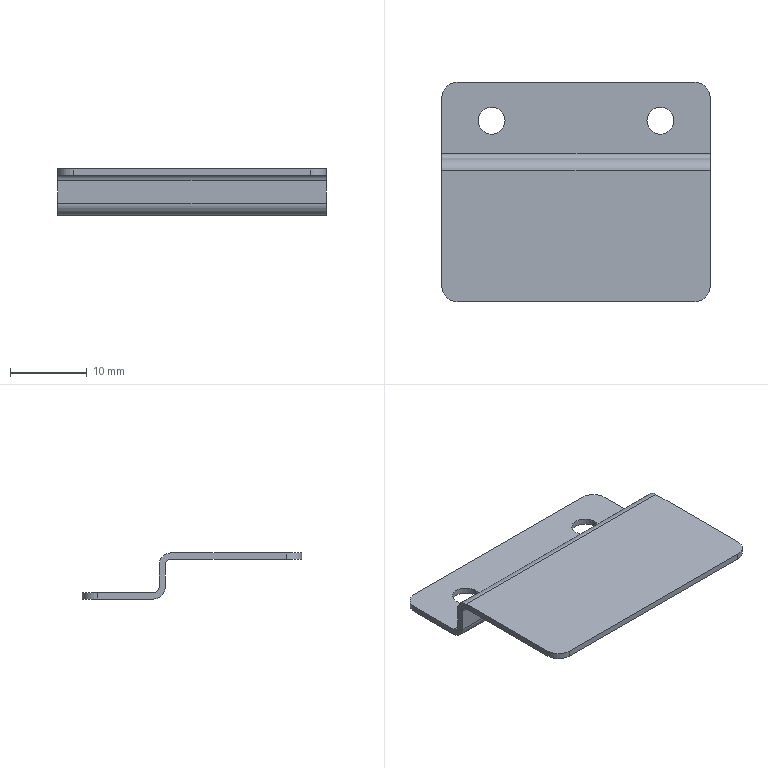Part | SolidWorks | features BaseBody 1 | 1 solid | 22 faces | box 35 x 28.6 x 6 mm | volume 900.941 mm3 | cylinder 12 | plane 10 | commonest cylinder face diameters 3.5 x4 4 x4 1.473 x2 3.073 x2
STEP:
#1=CARTESIAN_POINT('',(12.75,0.,0.8));
#2=VERTEX_POINT('',#1);
#3=CARTESIAN_POINT('',(9.25,0.,0.8));
#4=VERTEX_POINT('',#3);
#5=CARTESIAN_POINT('',(11.,0.,0.8));
#6=DIRECTION('',(0.,0.,-1.));
#7=DIRECTION('',(-1.,0.,0.));
#8=AXIS2_PLACEMENT_3D('',#5,#6,#7);
#9=CIRCLE('',#8,1.75);
#10=EDGE_CURVE('',#2,#4,#9,.T.);
#11=ORIENTED_EDGE('',*,*,#10,.F.);
#12=CARTESIAN_POINT('',(12.75,0.,0.));
#13=VERTEX_POINT('',#12);
#14=CARTESIAN_POINT('',(12.75,0.,0.8));
#15=DIRECTION('',(0.,0.,-1.));
#16=VECTOR('',#15,1000.);
#17=LINE('',#14,#16);
#18=EDGE_CURVE('',#2,#13,#17,.T.);
#19=ORIENTED_EDGE('',*,*,#18,.T.);
#20=CARTESIAN_POINT('',(9.25,0.,0.));
#21=VERTEX_POINT('',#20);
#22=CARTESIAN_POINT('',(11.,0.,0.));
#23=DIRECTION('',(0.,0.,1.));
#24=DIRECTION('',(-1.,0.,0.));
#25=AXIS2_PLACEMENT_3D('',#22,#23,#24);
#26=CIRCLE('',#25,1.75);
#27=EDGE_CURVE('',#21,#13,#26,.T.);
#28=ORIENTED_EDGE('',*,*,#27,.F.);
#29=CARTESIAN_POINT('',(9.25,0.,0.8));
#30=DIRECTION('',(0.,0.,-1.));
#31=VECTOR('',#30,1000.);
#32=LINE('',#29,#31);
#33=EDGE_CURVE('',#4,#21,#32,.T.);
#34=ORIENTED_EDGE('',*,*,#33,.F.);
#35=EDGE_LOOP('',(#11,#19,#28,#34));
#36=FACE_OUTER_BOUND('',#35,.T.);
#37=CARTESIAN_POINT('',(11.,0.,0.8));
#38=DIRECTION('',(0.,0.,-1.));
#39=DIRECTION('',(-1.,0.,0.));
#40=AXIS2_PLACEMENT_3D('',#37,#38,#39);
#41=CYLINDRICAL_SURFACE('',#40,1.75);
#42=ADVANCED_FACE('',(#36),#41,.F.);
#43=CARTESIAN_POINT('',(-9.25,0.,0.8));
#44=VERTEX_POINT('',#43);
#45=CARTESIAN_POINT('',(-12.75,0.,0.8));
#46=VERTEX_POINT('',#45);
#47=CARTESIAN_POINT('',(-11.,0.,0.8));
#48=DIRECTION('',(0.,0.,-1.));
#49=DIRECTION('',(-1.,0.,0.));
#50=AXIS2_PLACEMENT_3D('',#47,#48,#49);
#51=CIRCLE('',#50,1.75);
#52=EDGE_CURVE('',#44,#46,#51,.T.);
#53=ORIENTED_EDGE('',*,*,#52,.F.);
#54=CARTESIAN_POINT('',(-9.25,0.,0.));
#55=VERTEX_POINT('',#54);
#56=CARTESIAN_POINT('',(-9.25,0.,0.8));
#57=DIRECTION('',(0.,0.,-1.));
#58=VECTOR('',#57,1000.);
#59=LINE('',#56,#58);
#60=EDGE_CURVE('',#44,#55,#59,.T.);
#61=ORIENTED_EDGE('',*,*,#60,.T.);
#62=CARTESIAN_POINT('',(-12.75,0.,0.));
#63=VERTEX_POINT('',#62);
#64=CARTESIAN_POINT('',(-11.,0.,0.));
#65=DIRECTION('',(0.,0.,1.));
#66=DIRECTION('',(-1.,0.,0.));
#67=AXIS2_PLACEMENT_3D('',#64,#65,#66);
#68=CIRCLE('',#67,1.75);
#69=EDGE_CURVE('',#63,#55,#68,.T.);
#70=ORIENTED_EDGE('',*,*,#69,.F.);
#71=CARTESIAN_POINT('',(-12.75,0.,0.8));
#72=DIRECTION('',(0.,0.,-1.));
#73=VECTOR('',#72,1000.);
#74=LINE('',#71,#73);
#75=EDGE_CURVE('',#46,#63,#74,.T.);
#76=ORIENTED_EDGE('',*,*,#75,.F.);
#77=EDGE_LOOP('',(#53,#61,#70,#76));
#78=FACE_OUTER_BOUND('',#77,.T.);
#79=CARTESIAN_POINT('',(-11.,0.,0.8));
#80=DIRECTION('',(0.,0.,-1.));
#81=DIRECTION('',(-1.,0.,0.));
#82=AXIS2_PLACEMENT_3D('',#79,#80,#81);
#83=CYLINDRICAL_SURFACE('',#82,1.75);
#84=ADVANCED_FACE('',(#78),#83,.F.);
#85=CARTESIAN_POINT('',(-17.5,-6.537,6.));
#86=VERTEX_POINT('',#85);
#87=CARTESIAN_POINT('',(-17.5,-21.6,6.));
#88=VERTEX_POINT('',#87);
#89=CARTESIAN_POINT('',(-17.5,0.,6.));
#90=DIRECTION('',(0.,-1.,0.));
#91=VECTOR('',#90,1000.);
#92=LINE('',#89,#91);
#93=EDGE_CURVE('',#86,#88,#92,.T.);
#94=ORIENTED_EDGE('',*,*,#93,.T.);
#95=CARTESIAN_POINT('',(-15.5,-23.6,6.));
#96=VERTEX_POINT('',#95);
#97=CARTESIAN_POINT('',(-15.5,-21.6,6.));
#98=DIRECTION('',(0.,0.,1.));
#99=DIRECTION('',(0.,1.,0.));
#100=AXIS2_PLACEMENT_3D('',#97,#98,#99);
#101=CIRCLE('',#100,2.);
#102=EDGE_CURVE('',#88,#96,#101,.T.);
#103=ORIENTED_EDGE('',*,*,#102,.T.);
#104=CARTESIAN_POINT('',(15.5,-23.6,6.));
#105=VERTEX_POINT('',#104);
#106=CARTESIAN_POINT('',(0.,-23.6,6.));
#107=DIRECTION('',(1.,0.,0.));
#108=VECTOR('',#107,1000.);
#109=LINE('',#106,#108);
#110=EDGE_CURVE('',#96,#105,#109,.T.);
#111=ORIENTED_EDGE('',*,*,#110,.T.);
#112=CARTESIAN_POINT('',(17.5,-21.6,6.));
#113=VERTEX_POINT('',#112);
#114=CARTESIAN_POINT('',(15.5,-21.6,6.));
#115=DIRECTION('',(0.,0.,1.));
#116=DIRECTION('',(0.,1.,0.));
#117=AXIS2_PLACEMENT_3D('',#114,#115,#116);
#118=CIRCLE('',#117,2.);
#119=EDGE_CURVE('',#105,#113,#118,.T.);
#120=ORIENTED_EDGE('',*,*,#119,.T.);
#121=CARTESIAN_POINT('',(17.5,-6.537,6.));
#122=VERTEX_POINT('',#121);
#123=CARTESIAN_POINT('',(17.5,0.,6.));
#124=DIRECTION('',(0.,1.,0.));
#125=VECTOR('',#124,1000.);
#126=LINE('',#123,#125);
#127=EDGE_CURVE('',#113,#122,#126,.T.);
#128=ORIENTED_EDGE('',*,*,#127,.T.);
#129=CARTESIAN_POINT('',(0.,-6.537,6.));
#130=DIRECTION('',(-1.,0.,0.));
#131=VECTOR('',#130,1000.);
#132=LINE('',#129,#131);
#133=EDGE_CURVE('',#122,#86,#132,.T.);
#134=ORIENTED_EDGE('',*,*,#133,.T.);
#135=EDGE_LOOP('',(#94,#103,#111,#120,#128,#134));
#136=FACE_OUTER_BOUND('',#135,.T.);
#137=CARTESIAN_POINT('',(0.,0.,6.));
#138=DIRECTION('',(0.,0.,1.));
#139=DIRECTION('',(1.,0.,0.));
#140=AXIS2_PLACEMENT_3D('',#137,#138,#139);
#141=PLANE('',#140);
#142=ADVANCED_FACE('',(#136),#141,.T.);
#143=CARTESIAN_POINT('',(-17.5,-21.6,5.2));
#144=VERTEX_POINT('',#143);
#145=CARTESIAN_POINT('',(-15.5,-23.6,5.2));
#146=VERTEX_POINT('',#145);
#147=CARTESIAN_POINT('',(-15.5,-21.6,5.2));
#148=DIRECTION('',(0.,0.,1.));
#149=DIRECTION('',(0.,1.,0.));
#150=AXIS2_PLACEMENT_3D('',#147,#148,#149);
#151=CIRCLE('',#150,2.);
#152=EDGE_CURVE('',#144,#146,#151,.T.);
#153=ORIENTED_EDGE('',*,*,#152,.T.);
#154=CARTESIAN_POINT('',(-15.5,-23.6,6.));
#155=DIRECTION('',(0.,0.,1.));
#156=VECTOR('',#155,1000.);
#157=LINE('',#154,#156);
#158=EDGE_CURVE('',#146,#96,#157,.T.);
#159=ORIENTED_EDGE('',*,*,#158,.T.);
#160=ORIENTED_EDGE('',*,*,#102,.F.);
#161=CARTESIAN_POINT('',(-17.5,-21.6,6.));
#162=DIRECTION('',(0.,0.,-1.));
#163=VECTOR('',#162,1000.);
#164=LINE('',#161,#163);
#165=EDGE_CURVE('',#88,#144,#164,.T.);
#166=ORIENTED_EDGE('',*,*,#165,.T.);
#167=EDGE_LOOP('',(#153,#159,#160,#166));
#168=FACE_OUTER_BOUND('',#167,.T.);
#169=CARTESIAN_POINT('',(-15.5,-21.6,6.));
#170=DIRECTION('',(0.,0.,-1.));
#171=DIRECTION('',(0.,1.,0.));
#172=AXIS2_PLACEMENT_3D('',#169,#170,#171);
#173=CYLINDRICAL_SURFACE('',#172,2.);
#174=ADVANCED_FACE('',(#168),#173,.T.);
#175=ORIENTED_EDGE('',*,*,#93,.F.);
#176=CARTESIAN_POINT('',(-17.5,-5.,4.463));
#177=VERTEX_POINT('',#176);
#178=CARTESIAN_POINT('',(-17.5,-6.537,4.463));
#179=DIRECTION('',(1.,0.,0.));
#180=DIRECTION('',(0.,0.,1.));
#181=AXIS2_PLACEMENT_3D('',#178,#179,#180);
#182=CIRCLE('',#181,1.537);
#183=EDGE_CURVE('',#177,#86,#182,.T.);
#184=ORIENTED_EDGE('',*,*,#183,.F.);
#185=CARTESIAN_POINT('',(-17.5,-5.,1.537));
#186=VERTEX_POINT('',#185);
#187=CARTESIAN_POINT('',(-17.5,-5.,0.));
#188=DIRECTION('',(0.,0.,-1.));
#189=VECTOR('',#188,1000.);
#190=LINE('',#187,#189);
#191=EDGE_CURVE('',#177,#186,#190,.T.);
#192=ORIENTED_EDGE('',*,*,#191,.T.);
#193=CARTESIAN_POINT('',(-17.5,-4.263,0.8));
#194=VERTEX_POINT('',#193);
#195=CARTESIAN_POINT('',(-17.5,-4.263,1.537));
#196=DIRECTION('',(1.,0.,0.));
#197=DIRECTION('',(0.,0.,-1.));
#198=AXIS2_PLACEMENT_3D('',#195,#196,#197);
#199=CIRCLE('',#198,0.7366);
#200=EDGE_CURVE('',#186,#194,#199,.T.);
#201=ORIENTED_EDGE('',*,*,#200,.T.);
#202=CARTESIAN_POINT('',(-17.5,3.,0.8));
#203=VERTEX_POINT('',#202);
#204=CARTESIAN_POINT('',(-17.5,0.,0.8));
#205=DIRECTION('',(0.,-1.,0.));
#206=VECTOR('',#205,1000.);
#207=LINE('',#204,#206);
#208=EDGE_CURVE('',#203,#194,#207,.T.);
#209=ORIENTED_EDGE('',*,*,#208,.F.);
#210=CARTESIAN_POINT('',(-17.5,3.,0.));
#211=VERTEX_POINT('',#210);
#212=CARTESIAN_POINT('',(-17.5,3.,0.8));
#213=DIRECTION('',(0.,0.,1.));
#214=VECTOR('',#213,1000.);
#215=LINE('',#212,#214);
#216=EDGE_CURVE('',#211,#203,#215,.T.);
#217=ORIENTED_EDGE('',*,*,#216,.F.);
#218=CARTESIAN_POINT('',(-17.5,-4.263,0.));
#219=VERTEX_POINT('',#218);
#220=CARTESIAN_POINT('',(-17.5,5.,0.));
#221=DIRECTION('',(0.,1.,0.));
#222=VECTOR('',#221,1000.);
#223=LINE('',#220,#222);
#224=EDGE_CURVE('',#219,#211,#223,.T.);
#225=ORIENTED_EDGE('',*,*,#224,.F.);
#226=CARTESIAN_POINT('',(-17.5,-5.8,1.537));
#227=VERTEX_POINT('',#226);
#228=CARTESIAN_POINT('',(-17.5,-4.263,1.537));
#229=DIRECTION('',(1.,0.,0.));
#230=DIRECTION('',(0.,0.,-1.));
#231=AXIS2_PLACEMENT_3D('',#228,#229,#230);
#232=CIRCLE('',#231,1.537);
#233=EDGE_CURVE('',#227,#219,#232,.T.);
#234=ORIENTED_EDGE('',*,*,#233,.F.);
#235=CARTESIAN_POINT('',(-17.5,-5.8,4.463));
#236=VERTEX_POINT('',#235);
#237=CARTESIAN_POINT('',(-17.5,-5.8,6.));
#238=DIRECTION('',(0.,0.,1.));
#239=VECTOR('',#238,1000.);
#240=LINE('',#237,#239);
#241=EDGE_CURVE('',#227,#236,#240,.T.);
#242=ORIENTED_EDGE('',*,*,#241,.T.);
#243=CARTESIAN_POINT('',(-17.5,-6.537,5.2));
#244=VERTEX_POINT('',#243);
#245=CARTESIAN_POINT('',(-17.5,-6.537,4.463));
#246=DIRECTION('',(-1.,0.,0.));
#247=DIRECTION('',(0.,0.,1.));
#248=AXIS2_PLACEMENT_3D('',#245,#246,#247);
#249=CIRCLE('',#248,0.7366);
#250=EDGE_CURVE('',#244,#236,#249,.T.);
#251=ORIENTED_EDGE('',*,*,#250,.F.);
#252=CARTESIAN_POINT('',(-17.5,-5.8,5.2));
#253=DIRECTION('',(0.,-1.,0.));
#254=VECTOR('',#253,1000.);
#255=LINE('',#252,#254);
#256=EDGE_CURVE('',#244,#144,#255,.T.);
#257=ORIENTED_EDGE('',*,*,#256,.T.);
#258=ORIENTED_EDGE('',*,*,#165,.F.);
#259=EDGE_LOOP('',(#175,#184,#192,#201,#209,#217,#225,#234,#242,#251,#257,#258));
#260=FACE_OUTER_BOUND('',#259,.T.);
#261=CARTESIAN_POINT('',(-17.5,-5.8,6.));
#262=DIRECTION('',(-1.,0.,0.));
#263=DIRECTION('',(0.,0.,1.));
#264=AXIS2_PLACEMENT_3D('',#261,#262,#263);
#265=PLANE('',#264);
#266=ADVANCED_FACE('',(#260),#265,.T.);
#267=ORIENTED_EDGE('',*,*,#133,.F.);
#268=CARTESIAN_POINT('',(17.5,-5.,4.463));
#269=VERTEX_POINT('',#268);
#270=CARTESIAN_POINT('',(17.5,-6.537,4.463));
#271=DIRECTION('',(-1.,0.,0.));
#272=DIRECTION('',(0.,0.,1.));
#273=AXIS2_PLACEMENT_3D('',#270,#271,#272);
#274=CIRCLE('',#273,1.537);
#275=EDGE_CURVE('',#122,#269,#274,.T.);
#276=ORIENTED_EDGE('',*,*,#275,.T.);
#277=CARTESIAN_POINT('',(-17.5,-5.,4.463));
#278=DIRECTION('',(-1.,0.,0.));
#279=VECTOR('',#278,1000.);
#280=LINE('',#277,#279);
#281=EDGE_CURVE('',#269,#177,#280,.T.);
#282=ORIENTED_EDGE('',*,*,#281,.T.);
#283=ORIENTED_EDGE('',*,*,#183,.T.);
#284=EDGE_LOOP('',(#267,#276,#282,#283));
#285=FACE_OUTER_BOUND('',#284,.T.);
#286=CARTESIAN_POINT('',(-17.5,-6.537,4.463));
#287=DIRECTION('',(-1.,0.,0.));
#288=DIRECTION('',(0.,0.,1.));
#289=AXIS2_PLACEMENT_3D('',#286,#287,#288);
#290=CYLINDRICAL_SURFACE('',#289,1.537);
#291=ADVANCED_FACE('',(#285),#290,.T.);
#292=CARTESIAN_POINT('',(17.5,-21.6,5.2));
#293=VERTEX_POINT('',#292);
#294=CARTESIAN_POINT('',(17.5,-6.537,5.2));
#295=VERTEX_POINT('',#294);
#296=CARTESIAN_POINT('',(17.5,-23.6,5.2));
#297=DIRECTION('',(0.,1.,0.));
#298=VECTOR('',#297,1000.);
#299=LINE('',#296,#298);
#300=EDGE_CURVE('',#293,#295,#299,.T.);
#301=ORIENTED_EDGE('',*,*,#300,.T.);
#302=CARTESIAN_POINT('',(17.5,-5.8,4.463));
#303=VERTEX_POINT('',#302);
#304=CARTESIAN_POINT('',(17.5,-6.537,4.463));
#305=DIRECTION('',(-1.,0.,0.));
#306=DIRECTION('',(0.,0.,1.));
#307=AXIS2_PLACEMENT_3D('',#304,#305,#306);
#308=CIRCLE('',#307,0.7366);
#309=EDGE_CURVE('',#295,#303,#308,.T.);
#310=ORIENTED_EDGE('',*,*,#309,.T.);
#311=CARTESIAN_POINT('',(17.5,-5.8,1.537));
#312=VERTEX_POINT('',#311);
#313=CARTESIAN_POINT('',(17.5,-5.8,0.8));
#314=DIRECTION('',(0.,0.,-1.));
#315=VECTOR('',#314,1000.);
#316=LINE('',#313,#315);
#317=EDGE_CURVE('',#303,#312,#316,.T.);
#318=ORIENTED_EDGE('',*,*,#317,.T.);
#319=CARTESIAN_POINT('',(17.5,-4.263,0.));
#320=VERTEX_POINT('',#319);
#321=CARTESIAN_POINT('',(17.5,-4.263,1.537));
#322=DIRECTION('',(-1.,0.,0.));
#323=DIRECTION('',(0.,0.,-1.));
#324=AXIS2_PLACEMENT_3D('',#321,#322,#323);
#325=CIRCLE('',#324,1.537);
#326=EDGE_CURVE('',#320,#312,#325,.T.);
#327=ORIENTED_EDGE('',*,*,#326,.F.);
#328=CARTESIAN_POINT('',(17.5,3.,0.));
#329=VERTEX_POINT('',#328);
#330=CARTESIAN_POINT('',(17.5,5.,0.));
#331=DIRECTION('',(0.,-1.,0.));
#332=VECTOR('',#331,1000.);
#333=LINE('',#330,#332);
#334=EDGE_CURVE('',#329,#320,#333,.T.);
#335=ORIENTED_EDGE('',*,*,#334,.F.);
#336=CARTESIAN_POINT('',(17.5,3.,0.8));
#337=VERTEX_POINT('',#336);
#338=CARTESIAN_POINT('',(17.5,3.,0.8));
#339=DIRECTION('',(0.,0.,-1.));
#340=VECTOR('',#339,1000.);
#341=LINE('',#338,#340);
#342=EDGE_CURVE('',#337,#329,#341,.T.);
#343=ORIENTED_EDGE('',*,*,#342,.F.);
#344=CARTESIAN_POINT('',(17.5,-4.263,0.8));
#345=VERTEX_POINT('',#344);
#346=CARTESIAN_POINT('',(17.5,0.,0.8));
#347=DIRECTION('',(0.,1.,0.));
#348=VECTOR('',#347,1000.);
#349=LINE('',#346,#348);
#350=EDGE_CURVE('',#345,#337,#349,.T.);
#351=ORIENTED_EDGE('',*,*,#350,.F.);
#352=CARTESIAN_POINT('',(17.5,-5.,1.537));
#353=VERTEX_POINT('',#352);
#354=CARTESIAN_POINT('',(17.5,-4.263,1.537));
#355=DIRECTION('',(1.,0.,0.));
#356=DIRECTION('',(0.,0.,-1.));
#357=AXIS2_PLACEMENT_3D('',#354,#355,#356);
#358=CIRCLE('',#357,0.7366);
#359=EDGE_CURVE('',#353,#345,#358,.T.);
#360=ORIENTED_EDGE('',*,*,#359,.F.);
#361=CARTESIAN_POINT('',(17.5,-5.,0.));
#362=DIRECTION('',(0.,0.,1.));
#363=VECTOR('',#362,1000.);
#364=LINE('',#361,#363);
#365=EDGE_CURVE('',#353,#269,#364,.T.);
#366=ORIENTED_EDGE('',*,*,#365,.T.);
#367=ORIENTED_EDGE('',*,*,#275,.F.);
#368=ORIENTED_EDGE('',*,*,#127,.F.);
#369=CARTESIAN_POINT('',(17.5,-21.6,6.));
#370=DIRECTION('',(0.,0.,-1.));
#371=VECTOR('',#370,1000.);
#372=LINE('',#369,#371);
#373=EDGE_CURVE('',#113,#293,#372,.T.);
#374=ORIENTED_EDGE('',*,*,#373,.T.);
#375=EDGE_LOOP('',(#301,#310,#318,#327,#335,#343,#351,#360,#366,#367,#368,#374));
#376=FACE_OUTER_BOUND('',#375,.T.);
#377=CARTESIAN_POINT('',(17.5,-23.6,6.));
#378=DIRECTION('',(1.,0.,0.));
#379=DIRECTION('',(0.,0.,-1.));
#380=AXIS2_PLACEMENT_3D('',#377,#378,#379);
#381=PLANE('',#380);
#382=ADVANCED_FACE('',(#376),#381,.T.);
#383=CARTESIAN_POINT('',(15.5,-23.6,5.2));
#384=VERTEX_POINT('',#383);
#385=CARTESIAN_POINT('',(15.5,-21.6,5.2));
#386=DIRECTION('',(0.,0.,1.));
#387=DIRECTION('',(0.,1.,0.));
#388=AXIS2_PLACEMENT_3D('',#385,#386,#387);
#389=CIRCLE('',#388,2.);
#390=EDGE_CURVE('',#384,#293,#389,.T.);
#391=ORIENTED_EDGE('',*,*,#390,.T.);
#392=ORIENTED_EDGE('',*,*,#373,.F.);
#393=ORIENTED_EDGE('',*,*,#119,.F.);
#394=CARTESIAN_POINT('',(15.5,-23.6,6.));
#395=DIRECTION('',(0.,0.,-1.));
#396=VECTOR('',#395,1000.);
#397=LINE('',#394,#396);
#398=EDGE_CURVE('',#105,#384,#397,.T.);
#399=ORIENTED_EDGE('',*,*,#398,.T.);
#400=EDGE_LOOP('',(#391,#392,#393,#399));
#401=FACE_OUTER_BOUND('',#400,.T.);
#402=CARTESIAN_POINT('',(15.5,-21.6,6.));
#403=DIRECTION('',(0.,0.,-1.));
#404=DIRECTION('',(0.,1.,0.));
#405=AXIS2_PLACEMENT_3D('',#402,#403,#404);
#406=CYLINDRICAL_SURFACE('',#405,2.);
#407=ADVANCED_FACE('',(#401),#406,.T.);
#408=ORIENTED_EDGE('',*,*,#110,.F.);
#409=ORIENTED_EDGE('',*,*,#158,.F.);
#410=CARTESIAN_POINT('',(-17.5,-23.6,5.2));
#411=DIRECTION('',(1.,0.,0.));
#412=VECTOR('',#411,1000.);
#413=LINE('',#410,#412);
#414=EDGE_CURVE('',#146,#384,#413,.T.);
#415=ORIENTED_EDGE('',*,*,#414,.T.);
#416=ORIENTED_EDGE('',*,*,#398,.F.);
#417=EDGE_LOOP('',(#408,#409,#415,#416));
#418=FACE_OUTER_BOUND('',#417,.T.);
#419=CARTESIAN_POINT('',(-17.5,-23.6,6.));
#420=DIRECTION('',(0.,-1.,0.));
#421=DIRECTION('',(0.,0.,-1.));
#422=AXIS2_PLACEMENT_3D('',#419,#420,#421);
#423=PLANE('',#422);
#424=ADVANCED_FACE('',(#418),#423,.T.);
#425=ORIENTED_EDGE('',*,*,#390,.F.);
#426=ORIENTED_EDGE('',*,*,#414,.F.);
#427=ORIENTED_EDGE('',*,*,#152,.F.);
#428=ORIENTED_EDGE('',*,*,#256,.F.);
#429=CARTESIAN_POINT('',(0.,-6.537,5.2));
#430=DIRECTION('',(-1.,0.,0.));
#431=VECTOR('',#430,1000.);
#432=LINE('',#429,#431);
#433=EDGE_CURVE('',#295,#244,#432,.T.);
#434=ORIENTED_EDGE('',*,*,#433,.F.);
#435=ORIENTED_EDGE('',*,*,#300,.F.);
#436=EDGE_LOOP('',(#425,#426,#427,#428,#434,#435));
#437=FACE_OUTER_BOUND('',#436,.T.);
#438=CARTESIAN_POINT('',(0.,0.,5.2));
#439=DIRECTION('',(0.,0.,1.));
#440=DIRECTION('',(1.,0.,0.));
#441=AXIS2_PLACEMENT_3D('',#438,#439,#440);
#442=PLANE('',#441);
#443=ADVANCED_FACE('',(#437),#442,.F.);
#444=ORIENTED_EDGE('',*,*,#365,.F.);
#445=CARTESIAN_POINT('',(0.,-5.,1.537));
#446=DIRECTION('',(1.,0.,0.));
#447=VECTOR('',#446,1000.);
#448=LINE('',#445,#447);
#449=EDGE_CURVE('',#186,#353,#448,.T.);
#450=ORIENTED_EDGE('',*,*,#449,.F.);
#451=ORIENTED_EDGE('',*,*,#191,.F.);
#452=ORIENTED_EDGE('',*,*,#281,.F.);
#453=EDGE_LOOP('',(#444,#450,#451,#452));
#454=FACE_OUTER_BOUND('',#453,.T.);
#455=CARTESIAN_POINT('',(0.,-5.,0.));
#456=DIRECTION('',(0.,-1.,0.));
#457=DIRECTION('',(0.,0.,-1.));
#458=AXIS2_PLACEMENT_3D('',#455,#456,#457);
#459=PLANE('',#458);
#460=ADVANCED_FACE('',(#454),#459,.F.);
#461=ORIENTED_EDGE('',*,*,#309,.F.);
#462=ORIENTED_EDGE('',*,*,#433,.T.);
#463=ORIENTED_EDGE('',*,*,#250,.T.);
#464=CARTESIAN_POINT('',(-17.5,-5.8,4.463));
#465=DIRECTION('',(-1.,0.,0.));
#466=VECTOR('',#465,1000.);
#467=LINE('',#464,#466);
#468=EDGE_CURVE('',#303,#236,#467,.T.);
#469=ORIENTED_EDGE('',*,*,#468,.F.);
#470=EDGE_LOOP('',(#461,#462,#463,#469));
#471=FACE_OUTER_BOUND('',#470,.T.);
#472=CARTESIAN_POINT('',(-17.5,-6.537,4.463));
#473=DIRECTION('',(-1.,0.,0.));
#474=DIRECTION('',(0.,0.,1.));
#475=AXIS2_PLACEMENT_3D('',#472,#473,#474);
#476=CYLINDRICAL_SURFACE('',#475,0.7366);
#477=ADVANCED_FACE('',(#471),#476,.F.);
#478=ORIENTED_EDGE('',*,*,#200,.F.);
#479=ORIENTED_EDGE('',*,*,#449,.T.);
#480=ORIENTED_EDGE('',*,*,#359,.T.);
#481=CARTESIAN_POINT('',(17.5,-4.263,0.8));
#482=DIRECTION('',(1.,0.,0.));
#483=VECTOR('',#482,1000.);
#484=LINE('',#481,#483);
#485=EDGE_CURVE('',#194,#345,#484,.T.);
#486=ORIENTED_EDGE('',*,*,#485,.F.);
#487=EDGE_LOOP('',(#478,#479,#480,#486));
#488=FACE_OUTER_BOUND('',#487,.T.);
#489=CARTESIAN_POINT('',(17.5,-4.263,1.537));
#490=DIRECTION('',(1.,0.,0.));
#491=DIRECTION('',(0.,0.,-1.));
#492=AXIS2_PLACEMENT_3D('',#489,#490,#491);
#493=CYLINDRICAL_SURFACE('',#492,0.7366);
#494=ADVANCED_FACE('',(#488),#493,.F.);
#495=ORIENTED_EDGE('',*,*,#241,.F.);
#496=CARTESIAN_POINT('',(0.,-5.8,1.537));
#497=DIRECTION('',(1.,0.,0.));
#498=VECTOR('',#497,1000.);
#499=LINE('',#496,#498);
#500=EDGE_CURVE('',#227,#312,#499,.T.);
#501=ORIENTED_EDGE('',*,*,#500,.T.);
#502=ORIENTED_EDGE('',*,*,#317,.F.);
#503=ORIENTED_EDGE('',*,*,#468,.T.);
#504=EDGE_LOOP('',(#495,#501,#502,#503));
#505=FACE_OUTER_BOUND('',#504,.T.);
#506=CARTESIAN_POINT('',(0.,-5.8,0.));
#507=DIRECTION('',(0.,-1.,0.));
#508=DIRECTION('',(0.,0.,-1.));
#509=AXIS2_PLACEMENT_3D('',#506,#507,#508);
#510=PLANE('',#509);
#511=ADVANCED_FACE('',(#505),#510,.T.);
#512=ORIENTED_EDGE('',*,*,#208,.T.);
#513=ORIENTED_EDGE('',*,*,#485,.T.);
#514=ORIENTED_EDGE('',*,*,#350,.T.);
#515=CARTESIAN_POINT('',(15.5,5.,0.8));
#516=VERTEX_POINT('',#515);
#517=CARTESIAN_POINT('',(15.5,3.,0.8));
#518=DIRECTION('',(0.,0.,1.));
#519=DIRECTION('',(-1.,0.,0.));
#520=AXIS2_PLACEMENT_3D('',#517,#518,#519);
#521=CIRCLE('',#520,2.);
#522=EDGE_CURVE('',#337,#516,#521,.T.);
#523=ORIENTED_EDGE('',*,*,#522,.T.);
#524=CARTESIAN_POINT('',(-15.5,5.,0.8));
#525=VERTEX_POINT('',#524);
#526=CARTESIAN_POINT('',(0.,5.,0.8));
#527=DIRECTION('',(-1.,0.,0.));
#528=VECTOR('',#527,1000.);
#529=LINE('',#526,#528);
#530=EDGE_CURVE('',#516,#525,#529,.T.);
#531=ORIENTED_EDGE('',*,*,#530,.T.);
#532=CARTESIAN_POINT('',(-15.5,3.,0.8));
#533=DIRECTION('',(0.,0.,1.));
#534=DIRECTION('',(-1.,0.,0.));
#535=AXIS2_PLACEMENT_3D('',#532,#533,#534);
#536=CIRCLE('',#535,2.);
#537=EDGE_CURVE('',#525,#203,#536,.T.);
#538=ORIENTED_EDGE('',*,*,#537,.T.);
#539=EDGE_LOOP('',(#512,#513,#514,#523,#531,#538));
#540=FACE_OUTER_BOUND('',#539,.T.);
#541=CARTESIAN_POINT('',(11.,0.,0.8));
#542=DIRECTION('',(0.,0.,-1.));
#543=DIRECTION('',(-1.,0.,0.));
#544=AXIS2_PLACEMENT_3D('',#541,#542,#543);
#545=CIRCLE('',#544,1.75);
#546=EDGE_CURVE('',#4,#2,#545,.T.);
#547=ORIENTED_EDGE('',*,*,#546,.T.);
#548=ORIENTED_EDGE('',*,*,#10,.T.);
#549=EDGE_LOOP('',(#547,#548));
#550=FACE_BOUND('',#549,.T.);
#551=CARTESIAN_POINT('',(-11.,0.,0.8));
#552=DIRECTION('',(0.,0.,-1.));
#553=DIRECTION('',(-1.,0.,0.));
#554=AXIS2_PLACEMENT_3D('',#551,#552,#553);
#555=CIRCLE('',#554,1.75);
#556=EDGE_CURVE('',#46,#44,#555,.T.);
#557=ORIENTED_EDGE('',*,*,#556,.T.);
#558=ORIENTED_EDGE('',*,*,#52,.T.);
#559=EDGE_LOOP('',(#557,#558));
#560=FACE_BOUND('',#559,.T.);
#561=CARTESIAN_POINT('',(0.,0.,0.8));
#562=DIRECTION('',(0.,0.,1.));
#563=DIRECTION('',(1.,0.,0.));
#564=AXIS2_PLACEMENT_3D('',#561,#562,#563);
#565=PLANE('',#564);
#566=ADVANCED_FACE('',(#540,#550,#560),#565,.T.);
#567=ORIENTED_EDGE('',*,*,#500,.F.);
#568=ORIENTED_EDGE('',*,*,#233,.T.);
#569=CARTESIAN_POINT('',(17.5,-4.263,0.));
#570=DIRECTION('',(1.,0.,0.));
#571=VECTOR('',#570,1000.);
#572=LINE('',#569,#571);
#573=EDGE_CURVE('',#219,#320,#572,.T.);
#574=ORIENTED_EDGE('',*,*,#573,.T.);
#575=ORIENTED_EDGE('',*,*,#326,.T.);
#576=EDGE_LOOP('',(#567,#568,#574,#575));
#577=FACE_OUTER_BOUND('',#576,.T.);
#578=CARTESIAN_POINT('',(17.5,-4.263,1.537));
#579=DIRECTION('',(1.,0.,0.));
#580=DIRECTION('',(0.,0.,-1.));
#581=AXIS2_PLACEMENT_3D('',#578,#579,#580);
#582=CYLINDRICAL_SURFACE('',#581,1.537);
#583=ADVANCED_FACE('',(#577),#582,.T.);
#584=CARTESIAN_POINT('',(-15.5,5.,0.));
#585=VERTEX_POINT('',#584);
#586=CARTESIAN_POINT('',(-15.5,3.,0.));
#587=DIRECTION('',(0.,0.,1.));
#588=DIRECTION('',(-1.,0.,0.));
#589=AXIS2_PLACEMENT_3D('',#586,#587,#588);
#590=CIRCLE('',#589,2.);
#591=EDGE_CURVE('',#585,#211,#590,.T.);
#592=ORIENTED_EDGE('',*,*,#591,.T.);
#593=ORIENTED_EDGE('',*,*,#216,.T.);
#594=ORIENTED_EDGE('',*,*,#537,.F.);
#595=CARTESIAN_POINT('',(-15.5,5.,0.8));
#596=DIRECTION('',(0.,0.,-1.));
#597=VECTOR('',#596,1000.);
#598=LINE('',#595,#597);
#599=EDGE_CURVE('',#525,#585,#598,.T.);
#600=ORIENTED_EDGE('',*,*,#599,.T.);
#601=EDGE_LOOP('',(#592,#593,#594,#600));
#602=FACE_OUTER_BOUND('',#601,.T.);
#603=CARTESIAN_POINT('',(-15.5,3.,0.8));
#604=DIRECTION('',(0.,0.,-1.));
#605=DIRECTION('',(-1.,0.,0.));
#606=AXIS2_PLACEMENT_3D('',#603,#604,#605);
#607=CYLINDRICAL_SURFACE('',#606,2.);
#608=ADVANCED_FACE('',(#602),#607,.T.);
#609=CARTESIAN_POINT('',(15.5,5.,0.));
#610=VERTEX_POINT('',#609);
#611=CARTESIAN_POINT('',(15.5,5.,0.8));
#612=DIRECTION('',(0.,0.,1.));
#613=VECTOR('',#612,1000.);
#614=LINE('',#611,#613);
#615=EDGE_CURVE('',#610,#516,#614,.T.);
#616=ORIENTED_EDGE('',*,*,#615,.F.);
#617=CARTESIAN_POINT('',(-17.5,5.,0.));
#618=DIRECTION('',(1.,0.,0.));
#619=VECTOR('',#618,1000.);
#620=LINE('',#617,#619);
#621=EDGE_CURVE('',#585,#610,#620,.T.);
#622=ORIENTED_EDGE('',*,*,#621,.F.);
#623=ORIENTED_EDGE('',*,*,#599,.F.);
#624=ORIENTED_EDGE('',*,*,#530,.F.);
#625=EDGE_LOOP('',(#616,#622,#623,#624));
#626=FACE_OUTER_BOUND('',#625,.T.);
#627=CARTESIAN_POINT('',(-17.5,5.,0.8));
#628=DIRECTION('',(0.,-1.,0.));
#629=DIRECTION('',(0.,0.,-1.));
#630=AXIS2_PLACEMENT_3D('',#627,#628,#629);
#631=PLANE('',#630);
#632=ADVANCED_FACE('',(#626),#631,.F.);
#633=CARTESIAN_POINT('',(15.5,3.,0.));
#634=DIRECTION('',(0.,0.,1.));
#635=DIRECTION('',(-1.,0.,0.));
#636=AXIS2_PLACEMENT_3D('',#633,#634,#635);
#637=CIRCLE('',#636,2.);
#638=EDGE_CURVE('',#329,#610,#637,.T.);
#639=ORIENTED_EDGE('',*,*,#638,.T.);
#640=ORIENTED_EDGE('',*,*,#615,.T.);
#641=ORIENTED_EDGE('',*,*,#522,.F.);
#642=ORIENTED_EDGE('',*,*,#342,.T.);
#643=EDGE_LOOP('',(#639,#640,#641,#642));
#644=FACE_OUTER_BOUND('',#643,.T.);
#645=CARTESIAN_POINT('',(15.5,3.,0.8));
#646=DIRECTION('',(0.,0.,-1.));
#647=DIRECTION('',(-1.,0.,0.));
#648=AXIS2_PLACEMENT_3D('',#645,#646,#647);
#649=CYLINDRICAL_SURFACE('',#648,2.);
#650=ADVANCED_FACE('',(#644),#649,.T.);
#651=ORIENTED_EDGE('',*,*,#18,.F.);
#652=ORIENTED_EDGE('',*,*,#546,.F.);
#653=ORIENTED_EDGE('',*,*,#33,.T.);
#654=CARTESIAN_POINT('',(11.,0.,0.));
#655=DIRECTION('',(0.,0.,1.));
#656=DIRECTION('',(-1.,0.,0.));
#657=AXIS2_PLACEMENT_3D('',#654,#655,#656);
#658=CIRCLE('',#657,1.75);
#659=EDGE_CURVE('',#13,#21,#658,.T.);
#660=ORIENTED_EDGE('',*,*,#659,.F.);
#661=EDGE_LOOP('',(#651,#652,#653,#660));
#662=FACE_OUTER_BOUND('',#661,.T.);
#663=CARTESIAN_POINT('',(11.,0.,0.8));
#664=DIRECTION('',(0.,0.,-1.));
#665=DIRECTION('',(-1.,0.,0.));
#666=AXIS2_PLACEMENT_3D('',#663,#664,#665);
#667=CYLINDRICAL_SURFACE('',#666,1.75);
#668=ADVANCED_FACE('',(#662),#667,.F.);
#669=ORIENTED_EDGE('',*,*,#60,.F.);
#670=ORIENTED_EDGE('',*,*,#556,.F.);
#671=ORIENTED_EDGE('',*,*,#75,.T.);
#672=CARTESIAN_POINT('',(-11.,0.,0.));
#673=DIRECTION('',(0.,0.,1.));
#674=DIRECTION('',(-1.,0.,0.));
#675=AXIS2_PLACEMENT_3D('',#672,#673,#674);
#676=CIRCLE('',#675,1.75);
#677=EDGE_CURVE('',#55,#63,#676,.T.);
#678=ORIENTED_EDGE('',*,*,#677,.F.);
#679=EDGE_LOOP('',(#669,#670,#671,#678));
#680=FACE_OUTER_BOUND('',#679,.T.);
#681=CARTESIAN_POINT('',(-11.,0.,0.8));
#682=DIRECTION('',(0.,0.,-1.));
#683=DIRECTION('',(-1.,0.,0.));
#684=AXIS2_PLACEMENT_3D('',#681,#682,#683);
#685=CYLINDRICAL_SURFACE('',#684,1.75);
#686=ADVANCED_FACE('',(#680),#685,.F.);
#687=ORIENTED_EDGE('',*,*,#638,.F.);
#688=ORIENTED_EDGE('',*,*,#334,.T.);
#689=ORIENTED_EDGE('',*,*,#573,.F.);
#690=ORIENTED_EDGE('',*,*,#224,.T.);
#691=ORIENTED_EDGE('',*,*,#591,.F.);
#692=ORIENTED_EDGE('',*,*,#621,.T.);
#693=EDGE_LOOP('',(#687,#688,#689,#690,#691,#692));
#694=FACE_OUTER_BOUND('',#693,.T.);
#695=ORIENTED_EDGE('',*,*,#27,.T.);
#696=ORIENTED_EDGE('',*,*,#659,.T.);
#697=EDGE_LOOP('',(#695,#696));
#698=FACE_BOUND('',#697,.T.);
#699=ORIENTED_EDGE('',*,*,#69,.T.);
#700=ORIENTED_EDGE('',*,*,#677,.T.);
#701=EDGE_LOOP('',(#699,#700));
#702=FACE_BOUND('',#701,.T.);
#703=CARTESIAN_POINT('',(0.,0.,0.));
#704=DIRECTION('',(0.,0.,1.));
#705=DIRECTION('',(1.,0.,0.));
#706=AXIS2_PLACEMENT_3D('',#703,#704,#705);
#707=PLANE('',#706);
#708=ADVANCED_FACE('',(#694,#698,#702),#707,.F.);
#709=CLOSED_SHELL('',(#42,#84,#142,#174,#266,#291,#382,#407,#424,#443,#460,#477,#494,#511,#566,#583,#608,#632,#650,#668,#686,#708));
#710=MANIFOLD_SOLID_BREP('',#709);
#711=CARTESIAN_POINT('',(0.,0.,0.));
#712=DIRECTION('',(0.,0.,1.));
#713=DIRECTION('',(1.,0.,0.));
#714=AXIS2_PLACEMENT_3D('',#711,#712,#713);
#715=(LENGTH_UNIT()NAMED_UNIT(*)SI_UNIT(.MILLI.,.METRE.));
#716=UNCERTAINTY_MEASURE_WITH_UNIT(LENGTH_MEASURE(0.00001),#715,'','');
#717=(NAMED_UNIT(*)PLANE_ANGLE_UNIT()SI_UNIT($,.RADIAN.));
#718=(NAMED_UNIT(*)SI_UNIT($,.STERADIAN.)SOLID_ANGLE_UNIT());
#719=(GEOMETRIC_REPRESENTATION_CONTEXT(3)GLOBAL_UNCERTAINTY_ASSIGNED_CONTEXT((#716))GLOBAL_UNIT_ASSIGNED_CONTEXT((#715,#717,#718))REPRESENTATION_CONTEXT('',''));
#720=ADVANCED_BREP_SHAPE_REPRESENTATION('',(#710,#714),#719);